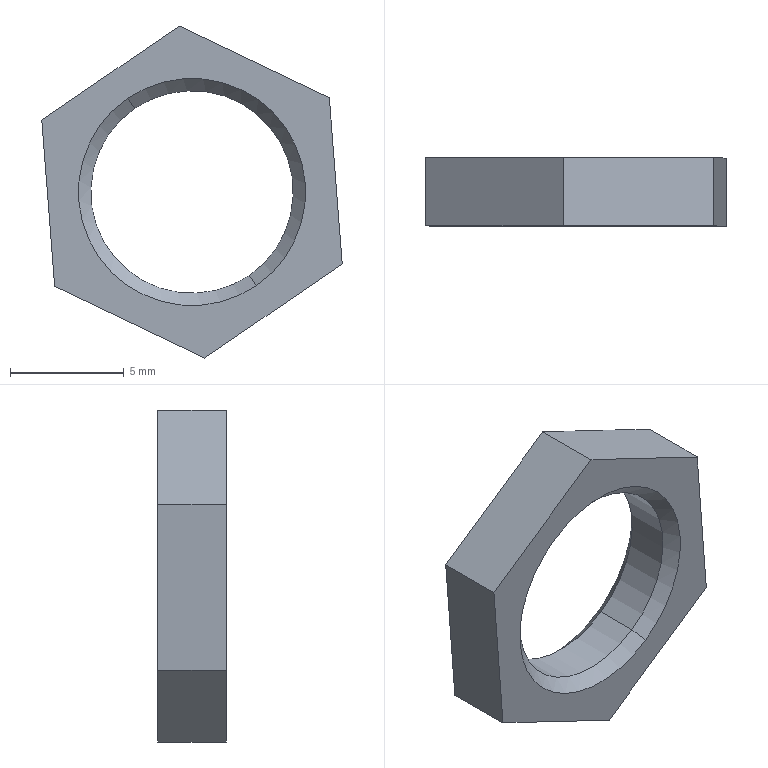Part | NX | features CONE_1 2 | 1 solid | 14 faces | box 13.228 x 3 x 14.621 mm | volume 223.149 mm3 | plane 8 | cone 4 | cylinder 2 | commonest cylinder face diameters 8.917 x2
STEP:
#1=CARTESIAN_POINT('',(-14.979,350.594,111.704));
#2=VERTEX_POINT('',#1);
#3=CARTESIAN_POINT('',(-20.021,350.594,119.059));
#4=VERTEX_POINT('',#3);
#5=CARTESIAN_POINT('',(-17.5,350.594,115.381));
#6=DIRECTION('',(0.,1.,0.));
#7=DIRECTION('',(-0.5654,0.,0.8248));
#8=AXIS2_PLACEMENT_3D('',#5,#6,#7);
#9=CIRCLE('',#8,4.458);
#10=EDGE_CURVE('',#2,#4,#9,.T.);
#11=ORIENTED_EDGE('',*,*,#10,.T.);
#12=CARTESIAN_POINT('',(-20.327,350.052,119.505));
#13=VERTEX_POINT('',#12);
#14=CARTESIAN_POINT('',(-20.327,350.052,119.505));
#15=DIRECTION('',(-0.3998,-0.7071,0.5833));
#16=VECTOR('',#15,1000.);
#17=LINE('',#14,#16);
#18=EDGE_CURVE('',#4,#13,#17,.T.);
#19=ORIENTED_EDGE('',*,*,#18,.T.);
#20=CARTESIAN_POINT('',(-14.673,350.052,111.257));
#21=VERTEX_POINT('',#20);
#22=CARTESIAN_POINT('',(-17.5,350.052,115.381));
#23=DIRECTION('',(0.,1.,0.));
#24=DIRECTION('',(-0.5654,0.,0.8248));
#25=AXIS2_PLACEMENT_3D('',#22,#23,#24);
#26=CIRCLE('',#25,5.);
#27=EDGE_CURVE('',#21,#13,#26,.T.);
#28=ORIENTED_EDGE('',*,*,#27,.F.);
#29=CARTESIAN_POINT('',(-14.673,350.052,111.257));
#30=DIRECTION('',(0.3998,-0.7071,-0.5833));
#31=VECTOR('',#30,1000.);
#32=LINE('',#29,#31);
#33=EDGE_CURVE('',#21,#2,#32,.F.);
#34=ORIENTED_EDGE('',*,*,#33,.T.);
#35=EDGE_LOOP('',(#11,#19,#28,#34));
#36=FACE_BOUND('',#35,.T.);
#37=CARTESIAN_POINT('',(-17.5,350.052,115.381));
#38=DIRECTION('',(0.,-1.,0.));
#39=DIRECTION('',(-0.5654,0.,0.8248));
#40=AXIS2_PLACEMENT_3D('',#37,#38,#39);
#41=CONICAL_SURFACE('',#40,5.,0.7854);
#42=ADVANCED_FACE('',(#36),#41,.F.);
#43=ORIENTED_EDGE('',*,*,#10,.F.);
#44=CARTESIAN_POINT('',(-14.979,352.511,111.704));
#45=VERTEX_POINT('',#44);
#46=CARTESIAN_POINT('',(-14.979,316.052,111.704));
#47=DIRECTION('',(0.,1.,0.));
#48=VECTOR('',#47,1000.);
#49=LINE('',#46,#48);
#50=EDGE_CURVE('',#2,#45,#49,.T.);
#51=ORIENTED_EDGE('',*,*,#50,.T.);
#52=CARTESIAN_POINT('',(-20.021,352.511,119.059));
#53=VERTEX_POINT('',#52);
#54=CARTESIAN_POINT('',(-17.5,352.511,115.381));
#55=DIRECTION('',(0.,1.,0.));
#56=DIRECTION('',(-0.5654,0.,0.8248));
#57=AXIS2_PLACEMENT_3D('',#54,#55,#56);
#58=CIRCLE('',#57,4.458);
#59=EDGE_CURVE('',#45,#53,#58,.T.);
#60=ORIENTED_EDGE('',*,*,#59,.T.);
#61=CARTESIAN_POINT('',(-20.021,316.052,119.059));
#62=DIRECTION('',(0.,1.,0.));
#63=VECTOR('',#62,1000.);
#64=LINE('',#61,#63);
#65=EDGE_CURVE('',#53,#4,#64,.F.);
#66=ORIENTED_EDGE('',*,*,#65,.T.);
#67=EDGE_LOOP('',(#43,#51,#60,#66));
#68=FACE_BOUND('',#67,.T.);
#69=CARTESIAN_POINT('',(-17.5,316.052,115.381));
#70=DIRECTION('',(0.,1.,0.));
#71=DIRECTION('',(0.5654,0.,-0.8248));
#72=AXIS2_PLACEMENT_3D('',#69,#70,#71);
#73=CYLINDRICAL_SURFACE('',#72,4.458);
#74=ADVANCED_FACE('',(#68),#73,.F.);
#75=ORIENTED_EDGE('',*,*,#59,.F.);
#76=CARTESIAN_POINT('',(-14.673,353.052,111.257));
#77=VERTEX_POINT('',#76);
#78=CARTESIAN_POINT('',(-14.979,352.511,111.704));
#79=DIRECTION('',(0.3998,0.7071,-0.5833));
#80=VECTOR('',#79,1000.);
#81=LINE('',#78,#80);
#82=EDGE_CURVE('',#45,#77,#81,.T.);
#83=ORIENTED_EDGE('',*,*,#82,.T.);
#84=CARTESIAN_POINT('',(-20.327,353.052,119.505));
#85=VERTEX_POINT('',#84);
#86=CARTESIAN_POINT('',(-17.5,353.052,115.381));
#87=DIRECTION('',(0.,1.,0.));
#88=DIRECTION('',(-0.5654,0.,0.8248));
#89=AXIS2_PLACEMENT_3D('',#86,#87,#88);
#90=CIRCLE('',#89,5.);
#91=EDGE_CURVE('',#77,#85,#90,.T.);
#92=ORIENTED_EDGE('',*,*,#91,.T.);
#93=CARTESIAN_POINT('',(-20.021,352.511,119.059));
#94=DIRECTION('',(-0.3998,0.7071,0.5833));
#95=VECTOR('',#94,1000.);
#96=LINE('',#93,#95);
#97=EDGE_CURVE('',#85,#53,#96,.F.);
#98=ORIENTED_EDGE('',*,*,#97,.T.);
#99=EDGE_LOOP('',(#75,#83,#92,#98));
#100=FACE_BOUND('',#99,.T.);
#101=CARTESIAN_POINT('',(-17.5,352.511,115.381));
#102=DIRECTION('',(0.,1.,0.));
#103=DIRECTION('',(0.5654,0.,-0.8248));
#104=AXIS2_PLACEMENT_3D('',#101,#102,#103);
#105=CONICAL_SURFACE('',#104,4.458,0.7854);
#106=ADVANCED_FACE('',(#100),#105,.F.);
#107=CARTESIAN_POINT('',(-10.886,353.052,112.216));
#108=VERTEX_POINT('',#107);
#109=CARTESIAN_POINT('',(-16.934,353.052,108.071));
#110=VERTEX_POINT('',#109);
#111=CARTESIAN_POINT('',(-10.886,353.052,112.216));
#112=DIRECTION('',(-0.8248,0.,-0.5654));
#113=VECTOR('',#112,1000.);
#114=LINE('',#111,#113);
#115=EDGE_CURVE('',#108,#110,#114,.T.);
#116=ORIENTED_EDGE('',*,*,#115,.F.);
#117=CARTESIAN_POINT('',(-10.886,350.052,112.216));
#118=VERTEX_POINT('',#117);
#119=CARTESIAN_POINT('',(-10.886,350.052,112.216));
#120=DIRECTION('',(0.,1.,0.));
#121=VECTOR('',#120,1000.);
#122=LINE('',#119,#121);
#123=EDGE_CURVE('',#118,#108,#122,.T.);
#124=ORIENTED_EDGE('',*,*,#123,.F.);
#125=CARTESIAN_POINT('',(-16.934,350.052,108.071));
#126=VERTEX_POINT('',#125);
#127=CARTESIAN_POINT('',(-10.886,350.052,112.216));
#128=DIRECTION('',(-0.8248,0.,-0.5654));
#129=VECTOR('',#128,1000.);
#130=LINE('',#127,#129);
#131=EDGE_CURVE('',#118,#126,#130,.T.);
#132=ORIENTED_EDGE('',*,*,#131,.T.);
#133=CARTESIAN_POINT('',(-16.934,350.052,108.071));
#134=DIRECTION('',(0.,1.,0.));
#135=VECTOR('',#134,1000.);
#136=LINE('',#133,#135);
#137=EDGE_CURVE('',#126,#110,#136,.T.);
#138=ORIENTED_EDGE('',*,*,#137,.T.);
#139=EDGE_LOOP('',(#116,#124,#132,#138));
#140=FACE_BOUND('',#139,.T.);
#141=CARTESIAN_POINT('',(-10.886,350.052,112.216));
#142=DIRECTION('',(0.5654,0.,-0.8248));
#143=DIRECTION('',(0.,-1.,0.));
#144=AXIS2_PLACEMENT_3D('',#141,#142,#143);
#145=PLANE('',#144);
#146=ADVANCED_FACE('',(#140),#145,.T.);
#147=CARTESIAN_POINT('',(-11.452,353.052,119.527));
#148=VERTEX_POINT('',#147);
#149=CARTESIAN_POINT('',(-11.452,353.052,119.527));
#150=DIRECTION('',(0.07719,0.,-0.997));
#151=VECTOR('',#150,1000.);
#152=LINE('',#149,#151);
#153=EDGE_CURVE('',#148,#108,#152,.T.);
#154=ORIENTED_EDGE('',*,*,#153,.F.);
#155=CARTESIAN_POINT('',(-11.452,350.052,119.527));
#156=VERTEX_POINT('',#155);
#157=CARTESIAN_POINT('',(-11.452,350.052,119.527));
#158=DIRECTION('',(0.,1.,0.));
#159=VECTOR('',#158,1000.);
#160=LINE('',#157,#159);
#161=EDGE_CURVE('',#156,#148,#160,.T.);
#162=ORIENTED_EDGE('',*,*,#161,.F.);
#163=CARTESIAN_POINT('',(-11.452,350.052,119.527));
#164=DIRECTION('',(0.07719,0.,-0.997));
#165=VECTOR('',#164,1000.);
#166=LINE('',#163,#165);
#167=EDGE_CURVE('',#156,#118,#166,.T.);
#168=ORIENTED_EDGE('',*,*,#167,.T.);
#169=ORIENTED_EDGE('',*,*,#123,.T.);
#170=EDGE_LOOP('',(#154,#162,#168,#169));
#171=FACE_BOUND('',#170,.T.);
#172=CARTESIAN_POINT('',(-11.452,350.052,119.527));
#173=DIRECTION('',(0.997,0.,0.07719));
#174=DIRECTION('',(-0.07719,0.,0.997));
#175=AXIS2_PLACEMENT_3D('',#172,#173,#174);
#176=PLANE('',#175);
#177=ADVANCED_FACE('',(#171),#176,.T.);
#178=CARTESIAN_POINT('',(-18.066,353.052,122.692));
#179=VERTEX_POINT('',#178);
#180=CARTESIAN_POINT('',(-18.066,353.052,122.692));
#181=DIRECTION('',(0.902,0.,-0.4317));
#182=VECTOR('',#181,1000.);
#183=LINE('',#180,#182);
#184=EDGE_CURVE('',#179,#148,#183,.T.);
#185=ORIENTED_EDGE('',*,*,#184,.F.);
#186=CARTESIAN_POINT('',(-18.066,350.052,122.692));
#187=VERTEX_POINT('',#186);
#188=CARTESIAN_POINT('',(-18.066,350.052,122.692));
#189=DIRECTION('',(0.,1.,0.));
#190=VECTOR('',#189,1000.);
#191=LINE('',#188,#190);
#192=EDGE_CURVE('',#187,#179,#191,.T.);
#193=ORIENTED_EDGE('',*,*,#192,.F.);
#194=CARTESIAN_POINT('',(-18.066,350.052,122.692));
#195=DIRECTION('',(0.902,0.,-0.4317));
#196=VECTOR('',#195,1000.);
#197=LINE('',#194,#196);
#198=EDGE_CURVE('',#187,#156,#197,.T.);
#199=ORIENTED_EDGE('',*,*,#198,.T.);
#200=ORIENTED_EDGE('',*,*,#161,.T.);
#201=EDGE_LOOP('',(#185,#193,#199,#200));
#202=FACE_BOUND('',#201,.T.);
#203=CARTESIAN_POINT('',(-18.066,350.052,122.692));
#204=DIRECTION('',(0.4317,0.,0.902));
#205=DIRECTION('',(-0.902,0.,0.4317));
#206=AXIS2_PLACEMENT_3D('',#203,#204,#205);
#207=PLANE('',#206);
#208=ADVANCED_FACE('',(#202),#207,.T.);
#209=CARTESIAN_POINT('',(-24.114,353.052,118.546));
#210=VERTEX_POINT('',#209);
#211=CARTESIAN_POINT('',(-24.114,353.052,118.546));
#212=DIRECTION('',(0.8248,0.,0.5654));
#213=VECTOR('',#212,1000.);
#214=LINE('',#211,#213);
#215=EDGE_CURVE('',#210,#179,#214,.T.);
#216=ORIENTED_EDGE('',*,*,#215,.F.);
#217=CARTESIAN_POINT('',(-24.114,350.052,118.546));
#218=VERTEX_POINT('',#217);
#219=CARTESIAN_POINT('',(-24.114,350.052,118.546));
#220=DIRECTION('',(0.,1.,0.));
#221=VECTOR('',#220,1000.);
#222=LINE('',#219,#221);
#223=EDGE_CURVE('',#218,#210,#222,.T.);
#224=ORIENTED_EDGE('',*,*,#223,.F.);
#225=CARTESIAN_POINT('',(-24.114,350.052,118.546));
#226=DIRECTION('',(0.8248,0.,0.5654));
#227=VECTOR('',#226,1000.);
#228=LINE('',#225,#227);
#229=EDGE_CURVE('',#218,#187,#228,.T.);
#230=ORIENTED_EDGE('',*,*,#229,.T.);
#231=ORIENTED_EDGE('',*,*,#192,.T.);
#232=EDGE_LOOP('',(#216,#224,#230,#231));
#233=FACE_BOUND('',#232,.T.);
#234=CARTESIAN_POINT('',(-24.114,350.052,118.546));
#235=DIRECTION('',(-0.5654,0.,0.8248));
#236=DIRECTION('',(0.,1.,0.));
#237=AXIS2_PLACEMENT_3D('',#234,#235,#236);
#238=PLANE('',#237);
#239=ADVANCED_FACE('',(#233),#238,.T.);
#240=CARTESIAN_POINT('',(-23.548,353.052,111.236));
#241=VERTEX_POINT('',#240);
#242=CARTESIAN_POINT('',(-23.548,353.052,111.236));
#243=DIRECTION('',(-0.07719,0.,0.997));
#244=VECTOR('',#243,1000.);
#245=LINE('',#242,#244);
#246=EDGE_CURVE('',#241,#210,#245,.T.);
#247=ORIENTED_EDGE('',*,*,#246,.F.);
#248=CARTESIAN_POINT('',(-23.548,350.052,111.236));
#249=VERTEX_POINT('',#248);
#250=CARTESIAN_POINT('',(-23.548,350.052,111.236));
#251=DIRECTION('',(0.,1.,0.));
#252=VECTOR('',#251,1000.);
#253=LINE('',#250,#252);
#254=EDGE_CURVE('',#249,#241,#253,.T.);
#255=ORIENTED_EDGE('',*,*,#254,.F.);
#256=CARTESIAN_POINT('',(-23.548,350.052,111.236));
#257=DIRECTION('',(-0.07719,0.,0.997));
#258=VECTOR('',#257,1000.);
#259=LINE('',#256,#258);
#260=EDGE_CURVE('',#249,#218,#259,.T.);
#261=ORIENTED_EDGE('',*,*,#260,.T.);
#262=ORIENTED_EDGE('',*,*,#223,.T.);
#263=EDGE_LOOP('',(#247,#255,#261,#262));
#264=FACE_BOUND('',#263,.T.);
#265=CARTESIAN_POINT('',(-23.548,350.052,111.236));
#266=DIRECTION('',(-0.997,0.,-0.07719));
#267=DIRECTION('',(0.07719,0.,-0.997));
#268=AXIS2_PLACEMENT_3D('',#265,#266,#267);
#269=PLANE('',#268);
#270=ADVANCED_FACE('',(#264),#269,.T.);
#271=CARTESIAN_POINT('',(-16.934,353.052,108.071));
#272=DIRECTION('',(-0.902,0.,0.4317));
#273=VECTOR('',#272,1000.);
#274=LINE('',#271,#273);
#275=EDGE_CURVE('',#110,#241,#274,.T.);
#276=ORIENTED_EDGE('',*,*,#275,.F.);
#277=ORIENTED_EDGE('',*,*,#137,.F.);
#278=CARTESIAN_POINT('',(-16.934,350.052,108.071));
#279=DIRECTION('',(-0.902,0.,0.4317));
#280=VECTOR('',#279,1000.);
#281=LINE('',#278,#280);
#282=EDGE_CURVE('',#126,#249,#281,.T.);
#283=ORIENTED_EDGE('',*,*,#282,.T.);
#284=ORIENTED_EDGE('',*,*,#254,.T.);
#285=EDGE_LOOP('',(#276,#277,#283,#284));
#286=FACE_BOUND('',#285,.T.);
#287=CARTESIAN_POINT('',(-16.934,350.052,108.071));
#288=DIRECTION('',(-0.4317,0.,-0.902));
#289=DIRECTION('',(0.902,0.,-0.4317));
#290=AXIS2_PLACEMENT_3D('',#287,#288,#289);
#291=PLANE('',#290);
#292=ADVANCED_FACE('',(#286),#291,.T.);
#293=ORIENTED_EDGE('',*,*,#27,.T.);
#294=CARTESIAN_POINT('',(-17.5,350.052,115.381));
#295=DIRECTION('',(0.,1.,0.));
#296=DIRECTION('',(-0.5654,0.,0.8248));
#297=AXIS2_PLACEMENT_3D('',#294,#295,#296);
#298=CIRCLE('',#297,5.);
#299=EDGE_CURVE('',#13,#21,#298,.T.);
#300=ORIENTED_EDGE('',*,*,#299,.T.);
#301=EDGE_LOOP('',(#293,#300));
#302=FACE_BOUND('',#301,.T.);
#303=ORIENTED_EDGE('',*,*,#131,.F.);
#304=ORIENTED_EDGE('',*,*,#167,.F.);
#305=ORIENTED_EDGE('',*,*,#198,.F.);
#306=ORIENTED_EDGE('',*,*,#229,.F.);
#307=ORIENTED_EDGE('',*,*,#260,.F.);
#308=ORIENTED_EDGE('',*,*,#282,.F.);
#309=EDGE_LOOP('',(#303,#304,#305,#306,#307,#308));
#310=FACE_BOUND('',#309,.T.);
#311=CARTESIAN_POINT('',(-17.5,350.052,115.381));
#312=DIRECTION('',(0.,1.,0.));
#313=DIRECTION('',(0.5654,0.,-0.8248));
#314=AXIS2_PLACEMENT_3D('',#311,#312,#313);
#315=PLANE('',#314);
#316=ADVANCED_FACE('',(#302,#310),#315,.F.);
#317=CARTESIAN_POINT('',(-17.5,353.052,115.381));
#318=DIRECTION('',(0.,1.,0.));
#319=DIRECTION('',(-0.5654,0.,0.8248));
#320=AXIS2_PLACEMENT_3D('',#317,#318,#319);
#321=CIRCLE('',#320,5.);
#322=EDGE_CURVE('',#85,#77,#321,.T.);
#323=ORIENTED_EDGE('',*,*,#322,.F.);
#324=ORIENTED_EDGE('',*,*,#91,.F.);
#325=EDGE_LOOP('',(#323,#324));
#326=FACE_BOUND('',#325,.T.);
#327=ORIENTED_EDGE('',*,*,#115,.T.);
#328=ORIENTED_EDGE('',*,*,#275,.T.);
#329=ORIENTED_EDGE('',*,*,#246,.T.);
#330=ORIENTED_EDGE('',*,*,#215,.T.);
#331=ORIENTED_EDGE('',*,*,#184,.T.);
#332=ORIENTED_EDGE('',*,*,#153,.T.);
#333=EDGE_LOOP('',(#327,#328,#329,#330,#331,#332));
#334=FACE_BOUND('',#333,.T.);
#335=CARTESIAN_POINT('',(-17.5,353.052,115.381));
#336=DIRECTION('',(0.,1.,0.));
#337=DIRECTION('',(0.5654,0.,-0.8248));
#338=AXIS2_PLACEMENT_3D('',#335,#336,#337);
#339=PLANE('',#338);
#340=ADVANCED_FACE('',(#326,#334),#339,.T.);
#341=ORIENTED_EDGE('',*,*,#82,.F.);
#342=CARTESIAN_POINT('',(-17.5,352.511,115.381));
#343=DIRECTION('',(0.,1.,0.));
#344=DIRECTION('',(-0.5654,0.,0.8248));
#345=AXIS2_PLACEMENT_3D('',#342,#343,#344);
#346=CIRCLE('',#345,4.458);
#347=EDGE_CURVE('',#53,#45,#346,.T.);
#348=ORIENTED_EDGE('',*,*,#347,.F.);
#349=ORIENTED_EDGE('',*,*,#97,.F.);
#350=ORIENTED_EDGE('',*,*,#322,.T.);
#351=EDGE_LOOP('',(#341,#348,#349,#350));
#352=FACE_BOUND('',#351,.T.);
#353=CARTESIAN_POINT('',(-17.5,352.511,115.381));
#354=DIRECTION('',(0.,1.,0.));
#355=DIRECTION('',(0.5654,0.,-0.8248));
#356=AXIS2_PLACEMENT_3D('',#353,#354,#355);
#357=CONICAL_SURFACE('',#356,4.458,0.7854);
#358=ADVANCED_FACE('',(#352),#357,.F.);
#359=ORIENTED_EDGE('',*,*,#50,.F.);
#360=CARTESIAN_POINT('',(-17.5,350.594,115.381));
#361=DIRECTION('',(0.,1.,0.));
#362=DIRECTION('',(-0.5654,0.,0.8248));
#363=AXIS2_PLACEMENT_3D('',#360,#361,#362);
#364=CIRCLE('',#363,4.458);
#365=EDGE_CURVE('',#4,#2,#364,.T.);
#366=ORIENTED_EDGE('',*,*,#365,.F.);
#367=ORIENTED_EDGE('',*,*,#65,.F.);
#368=ORIENTED_EDGE('',*,*,#347,.T.);
#369=EDGE_LOOP('',(#359,#366,#367,#368));
#370=FACE_BOUND('',#369,.T.);
#371=CARTESIAN_POINT('',(-17.5,316.052,115.381));
#372=DIRECTION('',(0.,1.,0.));
#373=DIRECTION('',(0.5654,0.,-0.8248));
#374=AXIS2_PLACEMENT_3D('',#371,#372,#373);
#375=CYLINDRICAL_SURFACE('',#374,4.458);
#376=ADVANCED_FACE('',(#370),#375,.F.);
#377=ORIENTED_EDGE('',*,*,#18,.F.);
#378=ORIENTED_EDGE('',*,*,#365,.T.);
#379=ORIENTED_EDGE('',*,*,#33,.F.);
#380=ORIENTED_EDGE('',*,*,#299,.F.);
#381=EDGE_LOOP('',(#377,#378,#379,#380));
#382=FACE_BOUND('',#381,.T.);
#383=CARTESIAN_POINT('',(-17.5,350.052,115.381));
#384=DIRECTION('',(0.,-1.,0.));
#385=DIRECTION('',(-0.5654,0.,0.8248));
#386=AXIS2_PLACEMENT_3D('',#383,#384,#385);
#387=CONICAL_SURFACE('',#386,5.,0.7854);
#388=ADVANCED_FACE('',(#382),#387,.F.);
#389=CLOSED_SHELL('',(#42,#74,#106,#146,#177,#208,#239,#270,#292,#316,#340,#358,#376,#388));
#390=MANIFOLD_SOLID_BREP('',#389);
#391=(LENGTH_UNIT()NAMED_UNIT(*)SI_UNIT(.MILLI.,.METRE.));
#392=UNCERTAINTY_MEASURE_WITH_UNIT(LENGTH_MEASURE(0.00001),#391,'','');
#393=(NAMED_UNIT(*)PLANE_ANGLE_UNIT()SI_UNIT($,.RADIAN.));
#394=(NAMED_UNIT(*)SI_UNIT($,.STERADIAN.)SOLID_ANGLE_UNIT());
#395=(GEOMETRIC_REPRESENTATION_CONTEXT(3)GLOBAL_UNCERTAINTY_ASSIGNED_CONTEXT((#392))GLOBAL_UNIT_ASSIGNED_CONTEXT((#391,#393,#394))REPRESENTATION_CONTEXT('',''));
#396=ADVANCED_BREP_SHAPE_REPRESENTATION('',(#390),#395);